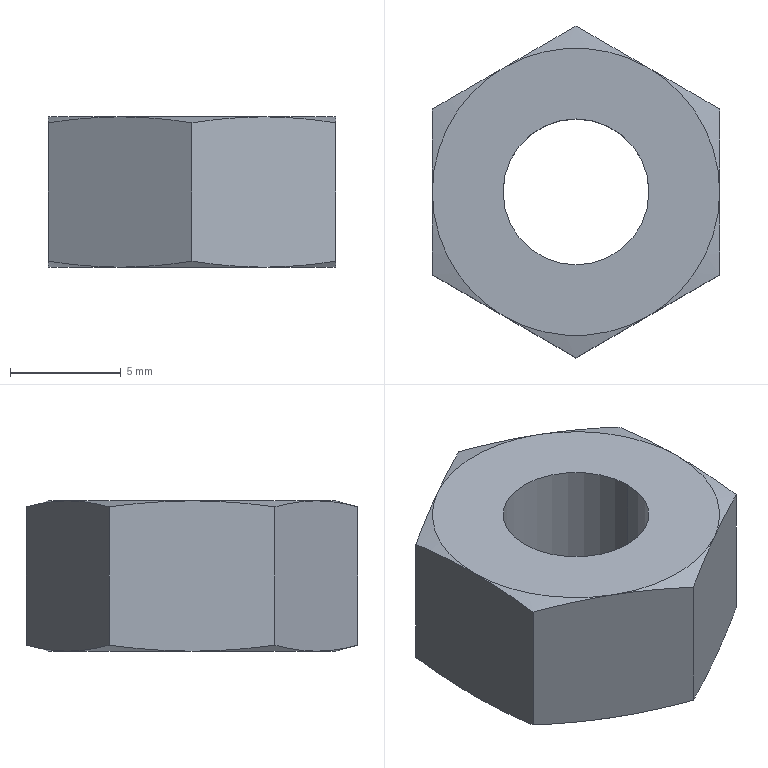Part | STEP file | 343.8-32-M8-63-A | 1 solid | 22 faces | box 13 x 15.011 x 6.8 mm | volume 760.328 mm3 | cone 12 | plane 8 | cylinder 2 | commonest cylinder face diameters 6.6 x2